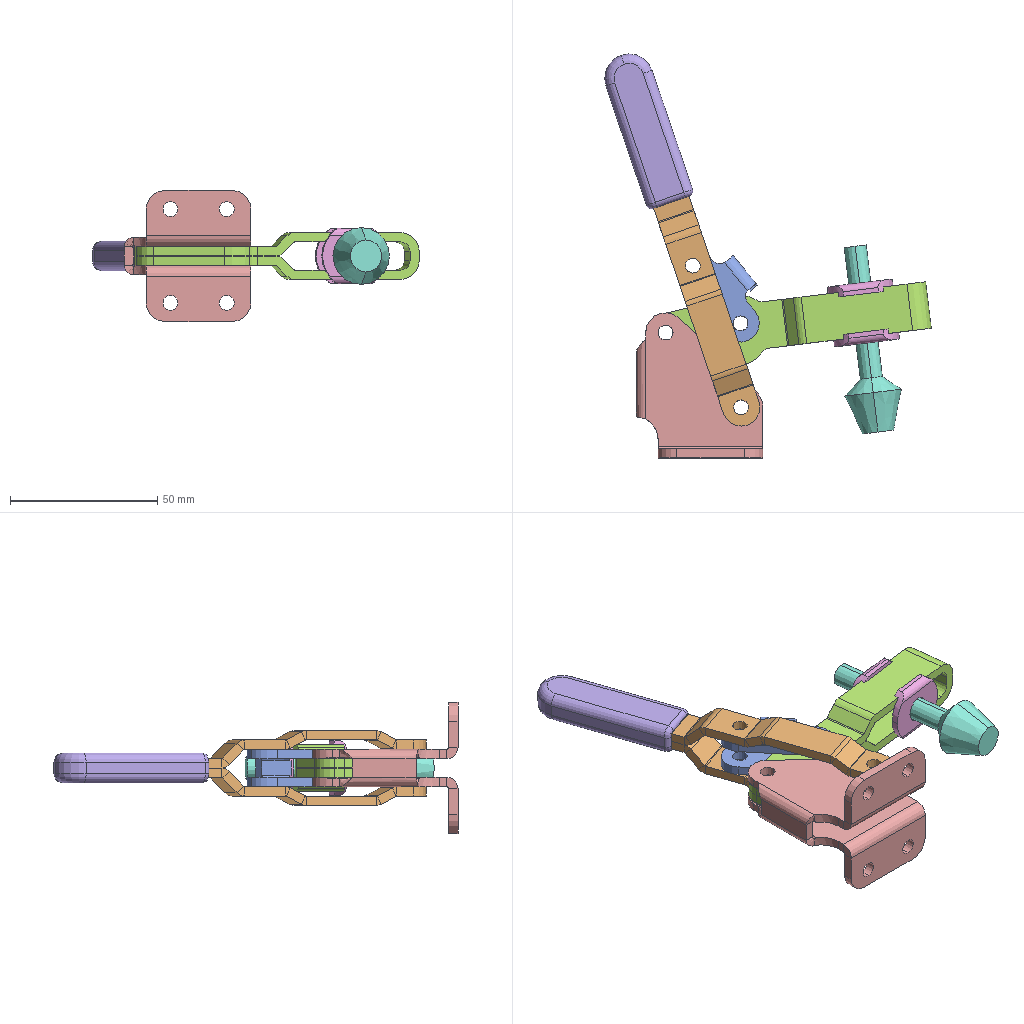Assembly | SolidWorks | 9 different items | 11 placed | box 111 x 137 x 44 mm
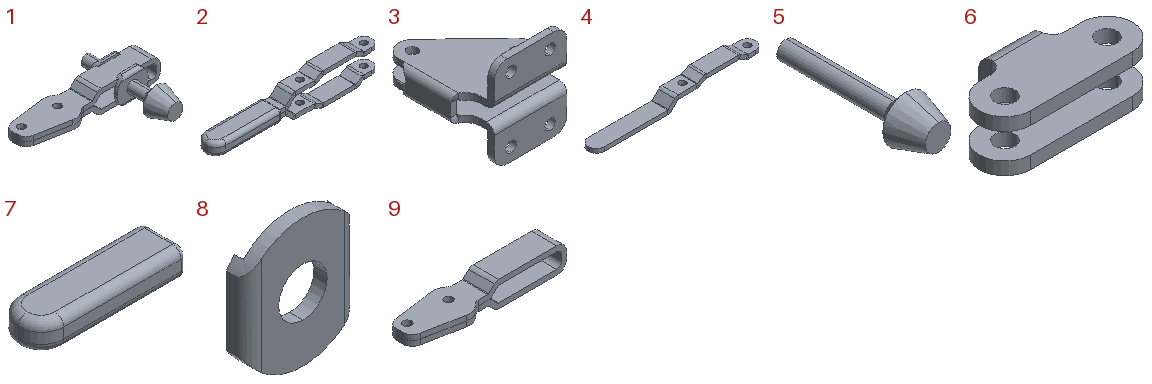Parts list (item | name | quantity | parent item | size | volume | features):
1 | (subassembly) | x1 | - | 96.012 x 63.5 x 19.304 mm | 17388 mm3 | -
2 | (subassembly) | x1 | - | 132.588 x 16.51 x 25.4 mm | 14412 mm3 | -
3 | - | x1 | - | 42.926 x 49.252 x 44.45 mm | 12813 mm3 | features Cut 5, Fillet 4, Boss 1, Extrusion 1, FlattenBends 1, ProcessBends 1, SheetMetal 1
4 | - | x2 | in 2 | 130.683 x 12.7 x 12.7 mm | 5187 mm3 | features Fillet 3, Cut 1, Extrusion 1, FlattenBends 1, ProcessBends 1, SheetMetal 1
5 | - | x1 | in 1 | 19.304 x 63.5 x 19.304 mm | 5277 mm3 | features Revolution 1
6 | - | x1 | - | 38.1 x 19.05 x 12.7 mm | 3299 mm3 | features Cut 3, Fillet 3, Boss 1, Extrusion 1
7 | - | x1 | in 2 | 52.705 x 16.51 x 10.16 mm | 4039 mm3 | features Fillet 3, Extrusion 1, Shell 1
8 | - | x2 | in 1 | 18.796 x 3.81 x 22.225 mm | 726.565 mm3 | features Boss 1, Cut 1, Extrusion 1, Fillet 1
9 | - | x1 | in 1 | 96.012 x 23.622 x 15.875 mm | 10658 mm3 | features Fillet 9, Cut 3, Boss 1, Extrusion 1
Mates (type | each side: item.copy, entity, surface, feature):
In the top assembly
Coincident | 3.1 face plane Base-Extrude | assembly plane | 3 times
Concentric | 3.1 face cylinder Cut-Extrude7 | 4.1 face cylinder Holes
Coincident | 3.1 face plane Base-Extrude | 4.1 face plane Base-Extrude
Concentric | 4.1 face cylinder Holes | 6.1 face cylinder Base-Extrude
Coincident | 4.1 face plane Base-Extrude | 6.1 face plane Base-Extrude
Concentric | 3.1 face cylinder Cut-Extrude7 | 9.1 face cylinder Cut-Extrude5
Coincident | 3.1 face plane Base-Extrude | 9.1 face plane Cut-Extrude1
Concentric | 9.1 face cylinder Cut-Extrude5 | 6.1 face cylinder Base-Extrude
In subassembly 2
Concentric | 4.2 face cylinder Holes | 4.3 face cylinder Holes | 2 times
Coincident | 4.2 face plane Base-Extrude | 4.3 face plane Base-Extrude
Coincident | 4.2 edge | 7.1 edge | 2 times
In subassembly 1
Parallel | 9.2 edge | 8.1 edge
Coincident | 9.2 face plane Base-Extrude | 8.1 face plane Base-Extrude
DistanceDim | 9.2 face plane Base-Extrude | 8.1 face plane Boss-Extrude1
Coincident | 9.2 face plane Base-Extrude | 8.2 face plane Base-Extrude
DistanceDim | 9.2 face plane Cut-Extrude1 | 5.1 plane
Concentric | 8.1 face cylinder Base-Extrude | 8.2 face cylinder Base-Extrude
Parallel | 8.1 edge | 8.2 face plane Cut-Extrude1
DistanceDim | 8.1 face plane Base-Extrude | 5.1 face plane Base-Revolve
Parallel | 8.2 face plane Base-Extrude | 5.1 face plane Base-Revolve
Concentric | 8.2 face cylinder Base-Extrude | 5.1 face cylinder Base-Revolve